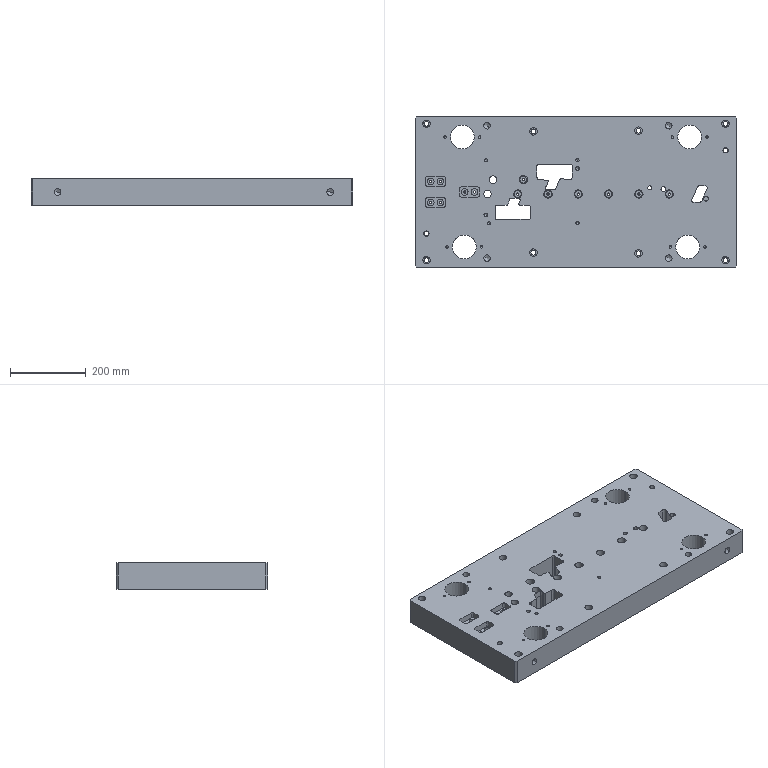Part | CATIA | 1 solid | 334 faces | box 850 x 400 x 70 mm | volume 21665405 mm3 | cylinder 195 | plane 70 | cone 48 | other 21 | commonest cylinder face diameters 6 x27 18 x26 13 x20 20 x20 6.8 x16 10 x16